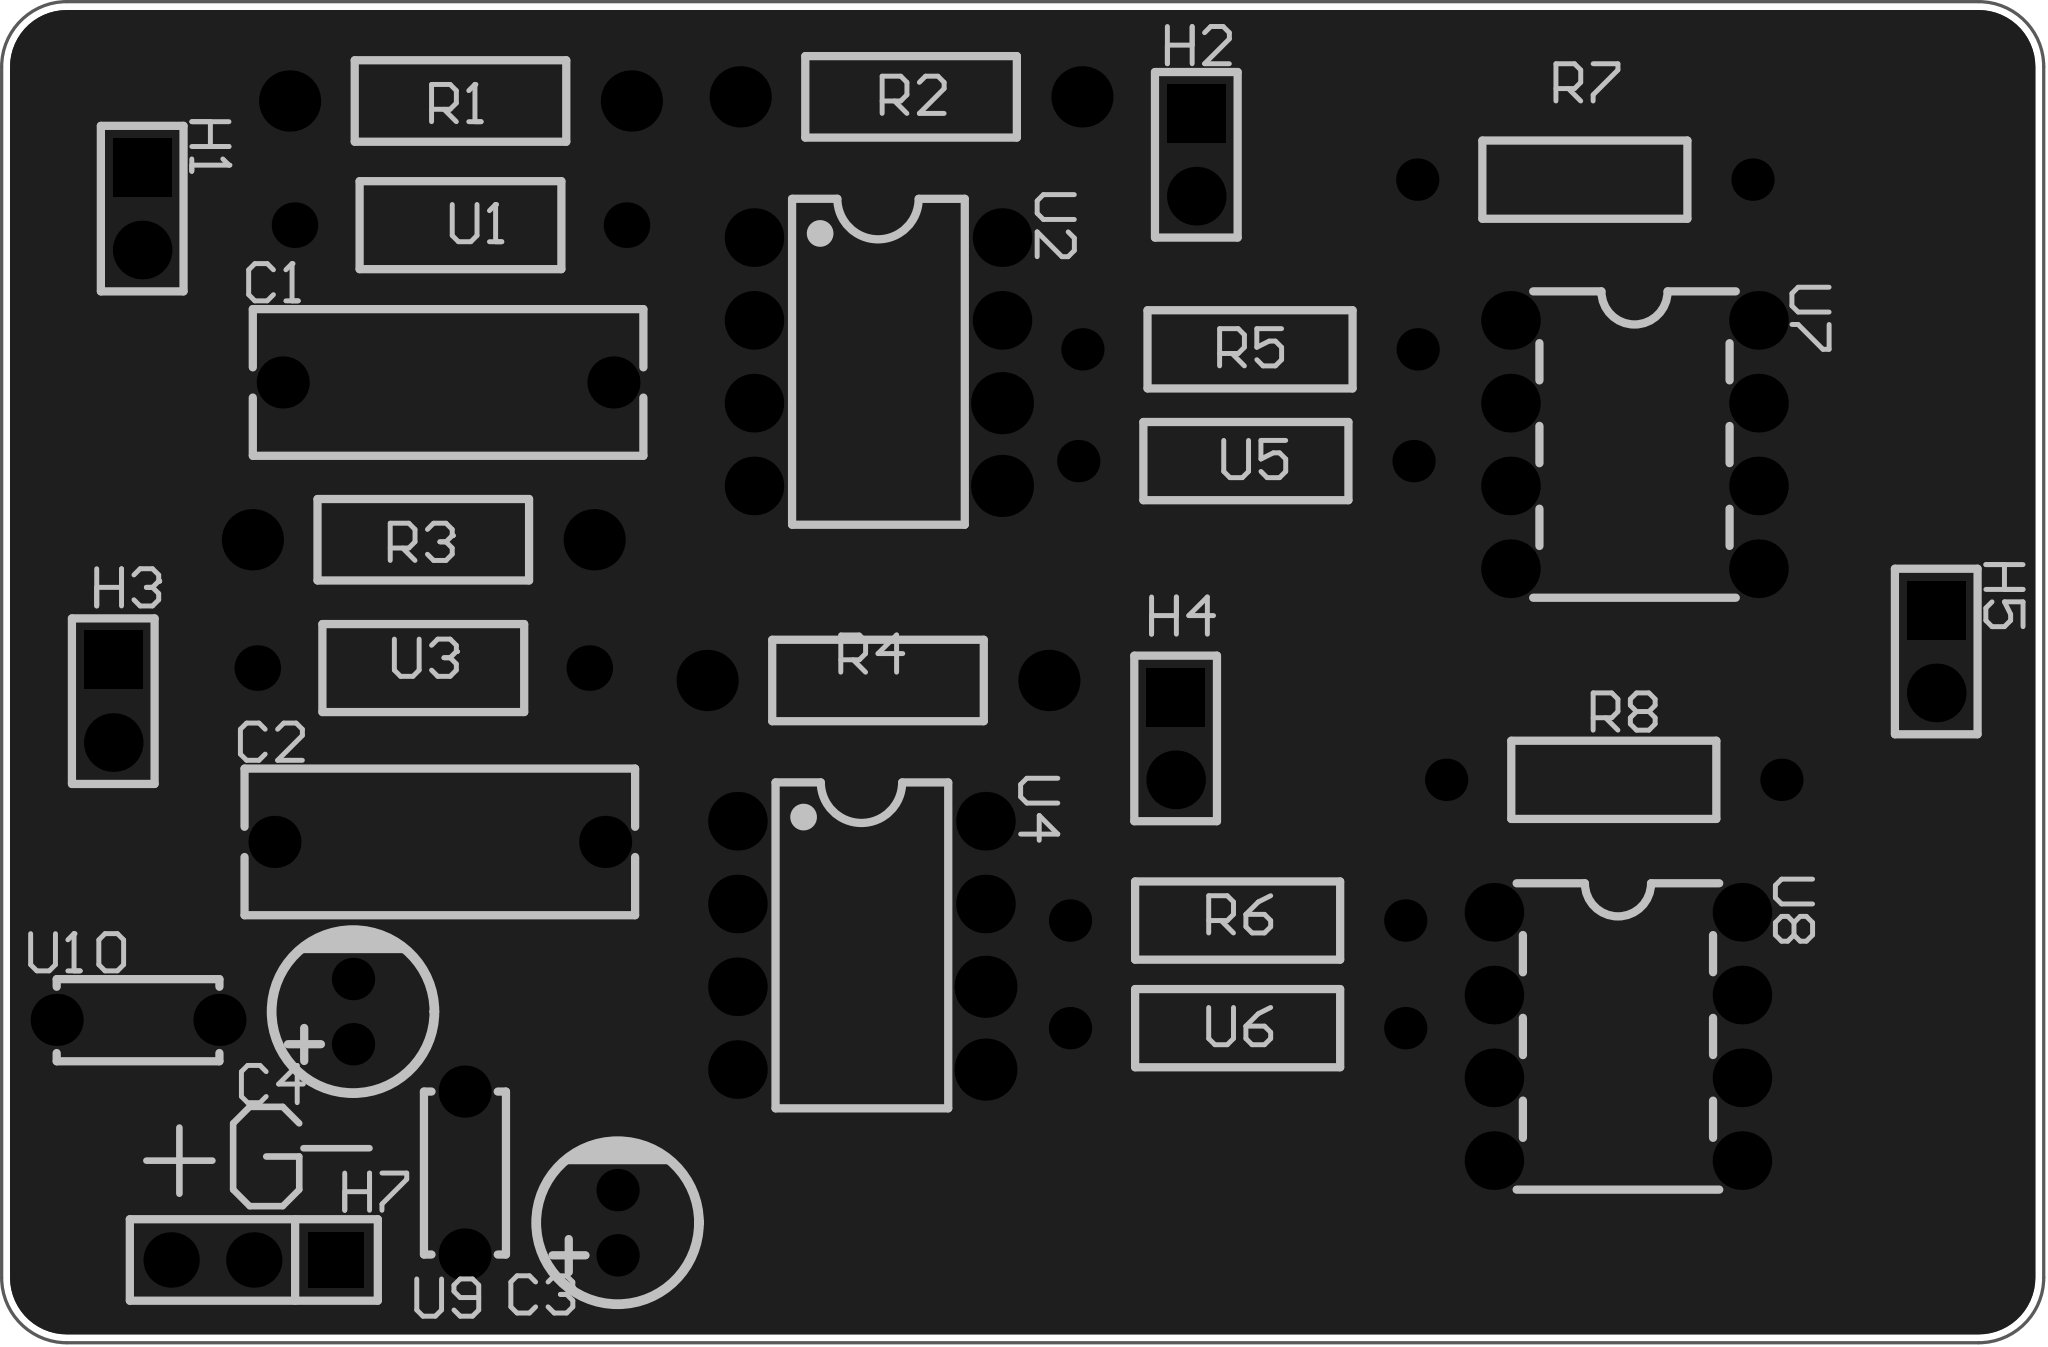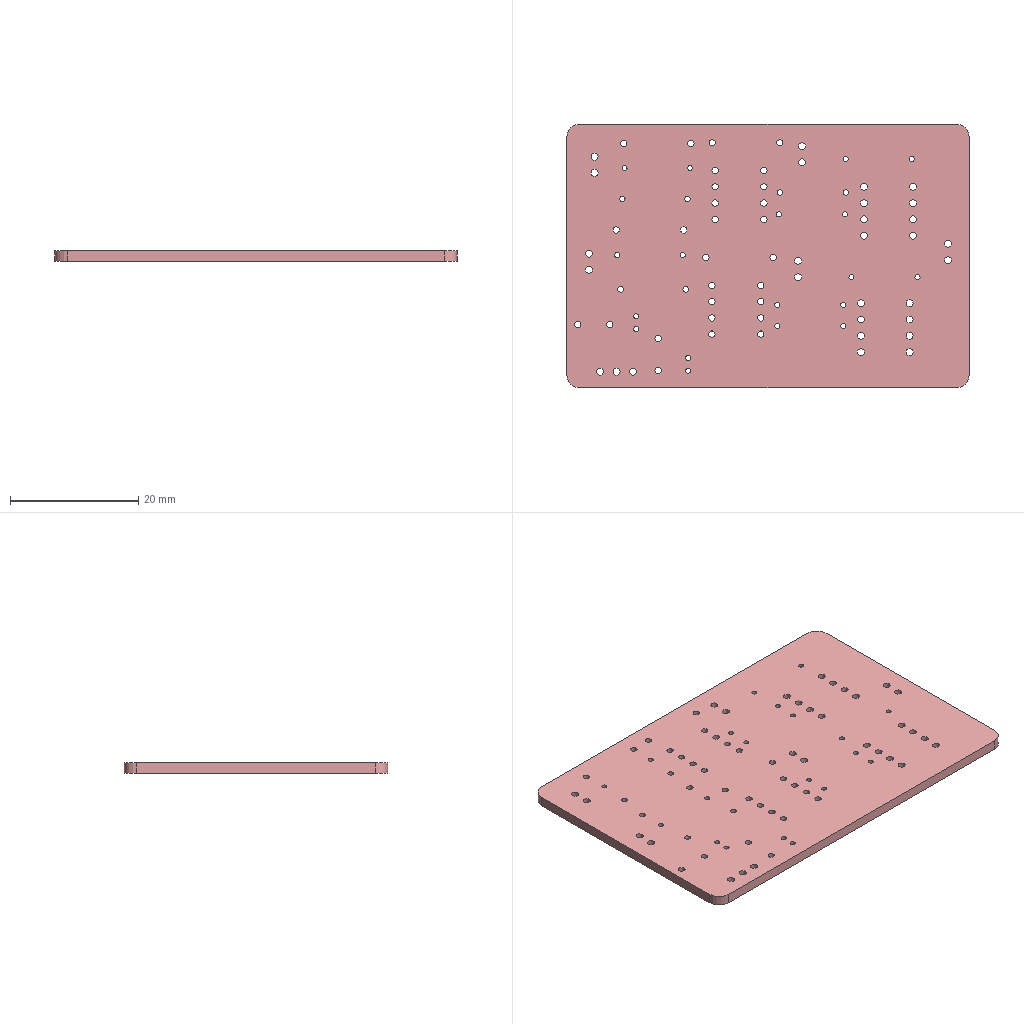Circuit board layout | Altium Designer | box 62.7 x 41.1 x 1.6 mm
Layer stack:
# Altium Designer layer stack of  (unit mm; dielectric type: 0 none, 1 core, 2 prepreg, 3 surface material)
index,name,kind,layer,copper_thickness_mm,dielectric_type,dielectric_thickness_mm,dielectric_material,dielectric_constant
0,Top Paste Mask Layer,other,,,,,,
1,Top Silkscreen Layer,other,,,,,,
2,Top Solder Mask Layer,dielectric,,,3,0.01,,3.3
3,Top Layer,copper,Top Layer,0.035,,,,
4,Dielectric1,dielectric,,,3,1.51,FR4,4.5
5,Bottom Layer,copper,Bottom Layer,0.035,,,,
6,Bottom Solder Mask Layer,dielectric,,,3,0.01,,3.3
7,Bottom Silkscreen Layer,other,,,,,,
8,Bottom Paste Mask Layer,other,,,,,,
# drill layer pairs: low layer,high layer
drill_pair,Top Layer,Bottom Layer
Part placement:
Designator,Comment,Layer,Footprint,Center-X(mm),Center-Y(mm),Rotation
C1,22nF,TopLayer,CAP-TH_L12.0-W4.5-P10.00-D1.0,93.218,108.839,0
C2,22nF,TopLayer,CAP-TH_L12.0-W4.5-P10.00-D1.0,92.964,94.742,0
H1,,TopLayer,HDR-TH_2P-P2.54-V-M-1,83.82,114.173,270
H2,,TopLayer,HDR-TH_2P-P2.54-V-M-1,116.205,115.824,270
H3,,TopLayer,HDR-TH_2P-P2.54-V-M-1,82.931,99.06,270
H4,,TopLayer,HDR-TH_2P-P2.54-V-M-1,115.57,97.917,270
H5,,TopLayer,HDR-TH_2P-P2.54-V-M-1,138.938,100.584,270
H7,,TopLayer,HDR-TH_3P-P2.54-V-M,87.249,81.915,180
R1,1kΩ,TopLayer,RES-TH_BD2.5-L6.5-P10.50-D0.6,93.599,117.475,0
R2,1kΩ,TopLayer,RES-TH_BD2.5-L6.5-P10.50-D0.6,107.442,117.602,0
R3,1kΩ,TopLayer,RES-TH_BD2.5-L6.5-P10.50-D0.6,92.456,104.013,0
R4,1kΩ,TopLayer,RES-TH_BD2.5-L6.5-P10.50-D0.6,106.426,99.695,0
R5,20kΩ,TopLayer,RES-TH_BD2.4-L6.3-P10.30-D0.6,117.856,109.855,0
R6,20kΩ,TopLayer,RES-TH_BD2.4-L6.3-P10.30-D0.6,117.475,92.329,0
R7,20kΩ,TopLayer,RES-TH_BD2.4-L6.3-P10.30-D0.6,128.143,115.062,0
R8,20kΩ,TopLayer,RES-TH_BD2.4-L6.3-P10.30-D0.6,129.032,96.647,0
U1,8.2kΩ,TopLayer,RES-TH_BD2.7-L6.2-P10.20-D0.4,93.599,113.665,0
U2,LF353N/NOPB,TopLayer,PDIP-8_L9.6-W6.4-P2.54-LS7.6-BL,106.426,109.474,270
U3,8.2kΩ,TopLayer,RES-TH_BD2.7-L6.2-P10.20-D0.4,92.456,100.076,0
U4,LF353N/NOPB,TopLayer,PDIP-8_L9.6-W6.4-P2.54-LS7.6-BL,105.918,91.567,270
U5,39kΩ,TopLayer,RES-TH_BD2.4-L6.3-P10.30-D0.6,117.729,106.426,0
U6,39kΩ,TopLayer,RES-TH_BD2.4-L6.3-P10.30-D0.6,117.475,89.027,0
U7,LM358N(XBLW),TopLayer,PDIP-8_L9.3-W6.4-P2.54-LS7.6-BL,129.667,106.934,270
U8,LM358N(XBLW),TopLayer,PDIP-8_L9.3-W6.4-P2.54-LS7.6-BL,129.159,88.773,270
C3,10uF,TopLayer,CAP-TH_BD5.0-P2.00-D0.8-FD-10UF50VC110GL,98.425,83.058,90
C4,10uF,TopLayer,CAP-TH_BD5.0-P2.00-D0.8-FD-10UF50VC110GL,90.297,89.535,90
U9,100nF,TopLayer,CAP-TH_L5.0-W2.5-P5.00-D1.0,93.726,84.582,90
U10,100nF,TopLayer,CAP-TH_L5.0-W2.5-P5.00-D1.0,83.693,89.281,0
Pad and via stacks:
# Altium Designer via and pad stacks of  (unit mm). Each distinct definition once, with the count of objects using it.
# via: kind,start_layer,end_layer,hole_mm,diameter_mm,mode(0 simple;1 top-mid-bottom;2 full stack),diameter_per_layer,count,example_net
# pad: kind,layer,hole_mm,hole_type(0 round;1 square;2 slot),plating,top_size,top_shape(1 round;2 rect;3 octagon;9 rounded rect),mid_size,bottom_size,mode,footprint,size_per_layer,count,example
pad,Multi-Layer,0.9,0,plated,1.6x1.6,1,1.6x1.6,1.6x1.6,0,CAP-TH_L12.0-W4.5-P10.00-D1.0,,4,C1.1
pad,Multi-Layer,1.1,0,plated,1.8x1.8,1,1.8x1.8,1.8x1.8,0,HDR-TH_2P-P2.54-V-M-1,,5,H1.2
pad,Multi-Layer,1.1,0,plated,1.8x1.8,2,1.8x1.8,1.8x1.8,0,HDR-TH_2P-P2.54-V-M-1,,5,H1.1
pad,Multi-Layer,1.1,0,plated,1.7x1.7,2,1.7x1.7,1.7x1.7,0,HDR-TH_3P-P2.54-V-M,,1,H7.1
pad,Multi-Layer,1.1,0,plated,1.7x1.7,1,1.7x1.7,1.7x1.7,0,HDR-TH_3P-P2.54-V-M,,2,H7.2
pad,Multi-Layer,1,0,plated,1.88x1.88,1,1.88x1.88,1.88x1.88,0,RES-TH_BD2.5-L6.5-P10.50-D0.6,,8,R1.1
pad,Multi-Layer,0.8,0,plated,1.3x1.3,1,1.3x1.3,1.3x1.3,0,RES-TH_BD2.4-L6.3-P10.30-D0.6,,12,R5.1
pad,Multi-Layer,0.8,0,plated,1.4x1.4,1,1.4x1.4,1.4x1.4,0,RES-TH_BD2.7-L6.2-P10.20-D0.4,,4,U1.1
pad,Multi-Layer,1,0,plated,1.8x1.8,1,1.8x1.8,1.8x1.8,0,PDIP-8_L9.6-W6.4-P2.54-LS7.6-BL,,12,U2.1
pad,Multi-Layer,1,0,plated,1.905x1.905,1,1.905x1.905,1.905x1.905,0,PDIP-8_L9.6-W6.4-P2.54-LS7.6-BL,,4,U2.5
pad,Multi-Layer,1.1,0,plated,1.8x1.8,1,1.8x1.8,1.8x1.8,0,PDIP-8_L9.3-W6.4-P2.54-LS7.6-BL,,16,U7.1
pad,Multi-Layer,0.8,0,plated,1.3x1.3,1,1.3x1.3,1.3x1.3,0,CAP-TH_BD5.0-P2.00-D0.8-FD-10UF50VC110GL,,4,C3.2
pad,Multi-Layer,1,0,plated,1.6x1.6,1,1.6x1.6,1.6x1.6,0,CAP-TH_L5.0-W2.5-P5.00-D1.0,,4,U9.1
Copper pours:
name,layer,net,type(0 solid;1 hatched;2 none)
Top Layer-GND,Top Layer,GND,0
Bottom Layer-GND,Bottom Layer,GND,0
Design rules, without the lines most boards share:
# Altium Designer design rules of  (exported by Altium Designer, unit mm)
# columns: name | kind | enabled | priority | scope1 | scope2 | descriptor | typed fields (field=value)
copperThickness2oz_2 | 2 | enabled | 1 | (InNet('+15V') OR InNet('-15V')) | All | Width Constraint (Min=8mil) (Max=100mil) (Preferred=43.3mil) ((InNet('+15V') OR InNet('-15V'))) |
copperThickness1oz_2 | 2 | enabled | 2 | All | All | Width Constraint (Min=5mil) (Max=100mil) (Preferred=13.8mil) (All) |